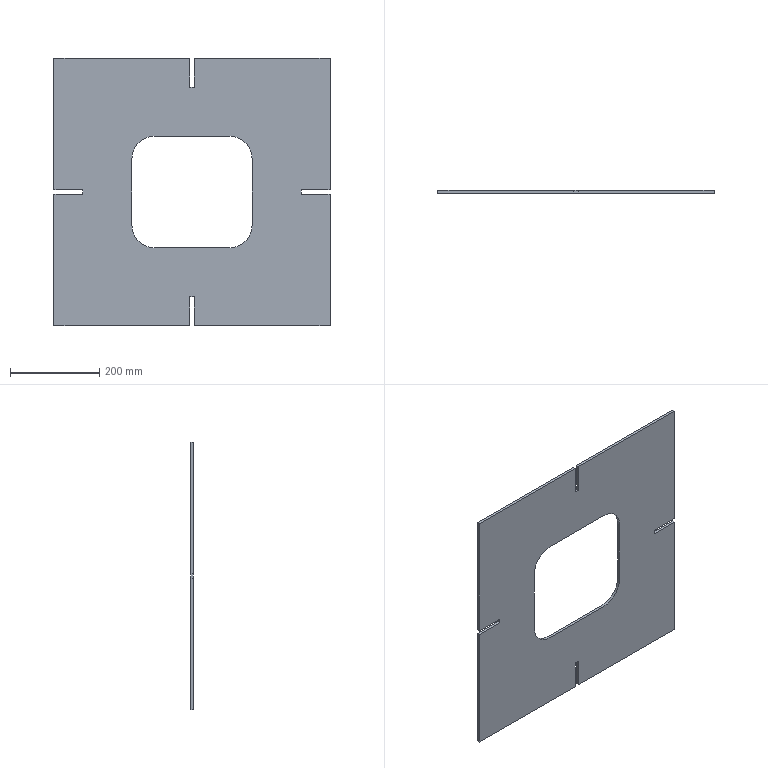Part | SolidWorks | features FlatPattern 1, SMBaseFlange 1, SheetMetal 1 | 1 solid | 30 faces | box 620 x 6 x 600 mm | volume 1824276 mm3 | plane 26 | cylinder 4 | commonest cylinder face diameters 100 x4
STEP:
#1=CARTESIAN_POINT('',(310.,0.,300.));
#2=VERTEX_POINT('',#1);
#3=CARTESIAN_POINT('',(310.,0.,5.));
#4=VERTEX_POINT('',#3);
#5=CARTESIAN_POINT('',(310.,0.,5.));
#6=DIRECTION('',(0.,0.,-1.));
#7=VECTOR('',#6,1000.);
#8=LINE('',#5,#7);
#9=EDGE_CURVE('',#2,#4,#8,.T.);
#10=ORIENTED_EDGE('',*,*,#9,.F.);
#11=CARTESIAN_POINT('',(310.,-6.,300.));
#12=VERTEX_POINT('',#11);
#13=CARTESIAN_POINT('',(310.,-6.,300.));
#14=DIRECTION('',(0.,1.,0.));
#15=VECTOR('',#14,1000.);
#16=LINE('',#13,#15);
#17=EDGE_CURVE('',#12,#2,#16,.T.);
#18=ORIENTED_EDGE('',*,*,#17,.F.);
#19=CARTESIAN_POINT('',(310.,-6.,5.));
#20=VERTEX_POINT('',#19);
#21=CARTESIAN_POINT('',(310.,-6.,5.));
#22=DIRECTION('',(0.,0.,-1.));
#23=VECTOR('',#22,1000.);
#24=LINE('',#21,#23);
#25=EDGE_CURVE('',#12,#20,#24,.T.);
#26=ORIENTED_EDGE('',*,*,#25,.T.);
#27=CARTESIAN_POINT('',(310.,-6.,5.));
#28=DIRECTION('',(0.,1.,0.));
#29=VECTOR('',#28,1000.);
#30=LINE('',#27,#29);
#31=EDGE_CURVE('',#20,#4,#30,.T.);
#32=ORIENTED_EDGE('',*,*,#31,.T.);
#33=EDGE_LOOP('',(#10,#18,#26,#32));
#34=FACE_OUTER_BOUND('',#33,.T.);
#35=CARTESIAN_POINT('',(310.,-6.,5.));
#36=DIRECTION('',(1.,0.,0.));
#37=DIRECTION('',(0.,0.,-1.));
#38=AXIS2_PLACEMENT_3D('',#35,#36,#37);
#39=PLANE('',#38);
#40=ADVANCED_FACE('',(#34),#39,.T.);
#41=CARTESIAN_POINT('',(5.,0.,300.));
#42=VERTEX_POINT('',#41);
#43=CARTESIAN_POINT('',(5.,0.,300.));
#44=DIRECTION('',(1.,0.,0.));
#45=VECTOR('',#44,1000.);
#46=LINE('',#43,#45);
#47=EDGE_CURVE('',#42,#2,#46,.T.);
#48=ORIENTED_EDGE('',*,*,#47,.F.);
#49=CARTESIAN_POINT('',(5.,-6.,300.));
#50=VERTEX_POINT('',#49);
#51=CARTESIAN_POINT('',(5.,-6.,300.));
#52=DIRECTION('',(0.,1.,0.));
#53=VECTOR('',#52,1000.);
#54=LINE('',#51,#53);
#55=EDGE_CURVE('',#50,#42,#54,.T.);
#56=ORIENTED_EDGE('',*,*,#55,.F.);
#57=CARTESIAN_POINT('',(5.,-6.,300.));
#58=DIRECTION('',(1.,0.,0.));
#59=VECTOR('',#58,1000.);
#60=LINE('',#57,#59);
#61=EDGE_CURVE('',#50,#12,#60,.T.);
#62=ORIENTED_EDGE('',*,*,#61,.T.);
#63=ORIENTED_EDGE('',*,*,#17,.T.);
#64=EDGE_LOOP('',(#48,#56,#62,#63));
#65=FACE_OUTER_BOUND('',#64,.T.);
#66=CARTESIAN_POINT('',(5.,-6.,300.));
#67=DIRECTION('',(0.,0.,1.));
#68=DIRECTION('',(1.,0.,0.));
#69=AXIS2_PLACEMENT_3D('',#66,#67,#68);
#70=PLANE('',#69);
#71=ADVANCED_FACE('',(#65),#70,.T.);
#72=CARTESIAN_POINT('',(5.,0.,235.));
#73=VERTEX_POINT('',#72);
#74=CARTESIAN_POINT('',(5.,0.,300.));
#75=DIRECTION('',(0.,0.,1.));
#76=VECTOR('',#75,1000.);
#77=LINE('',#74,#76);
#78=EDGE_CURVE('',#73,#42,#77,.T.);
#79=ORIENTED_EDGE('',*,*,#78,.F.);
#80=CARTESIAN_POINT('',(5.,-6.,235.));
#81=VERTEX_POINT('',#80);
#82=CARTESIAN_POINT('',(5.,-6.,235.));
#83=DIRECTION('',(0.,1.,0.));
#84=VECTOR('',#83,1000.);
#85=LINE('',#82,#84);
#86=EDGE_CURVE('',#81,#73,#85,.T.);
#87=ORIENTED_EDGE('',*,*,#86,.F.);
#88=CARTESIAN_POINT('',(5.,-6.,300.));
#89=DIRECTION('',(0.,0.,1.));
#90=VECTOR('',#89,1000.);
#91=LINE('',#88,#90);
#92=EDGE_CURVE('',#81,#50,#91,.T.);
#93=ORIENTED_EDGE('',*,*,#92,.T.);
#94=ORIENTED_EDGE('',*,*,#55,.T.);
#95=EDGE_LOOP('',(#79,#87,#93,#94));
#96=FACE_OUTER_BOUND('',#95,.T.);
#97=CARTESIAN_POINT('',(5.,-6.,300.));
#98=DIRECTION('',(-1.,0.,0.));
#99=DIRECTION('',(0.,0.,1.));
#100=AXIS2_PLACEMENT_3D('',#97,#98,#99);
#101=PLANE('',#100);
#102=ADVANCED_FACE('',(#96),#101,.T.);
#103=CARTESIAN_POINT('',(-5.,0.,235.));
#104=VERTEX_POINT('',#103);
#105=CARTESIAN_POINT('',(5.,0.,235.));
#106=DIRECTION('',(1.,0.,0.));
#107=VECTOR('',#106,1000.);
#108=LINE('',#105,#107);
#109=EDGE_CURVE('',#104,#73,#108,.T.);
#110=ORIENTED_EDGE('',*,*,#109,.F.);
#111=CARTESIAN_POINT('',(-5.,-6.,235.));
#112=VERTEX_POINT('',#111);
#113=CARTESIAN_POINT('',(-5.,-6.,235.));
#114=DIRECTION('',(0.,1.,0.));
#115=VECTOR('',#114,1000.);
#116=LINE('',#113,#115);
#117=EDGE_CURVE('',#112,#104,#116,.T.);
#118=ORIENTED_EDGE('',*,*,#117,.F.);
#119=CARTESIAN_POINT('',(5.,-6.,235.));
#120=DIRECTION('',(1.,0.,0.));
#121=VECTOR('',#120,1000.);
#122=LINE('',#119,#121);
#123=EDGE_CURVE('',#112,#81,#122,.T.);
#124=ORIENTED_EDGE('',*,*,#123,.T.);
#125=ORIENTED_EDGE('',*,*,#86,.T.);
#126=EDGE_LOOP('',(#110,#118,#124,#125));
#127=FACE_OUTER_BOUND('',#126,.T.);
#128=CARTESIAN_POINT('',(5.,-6.,235.));
#129=DIRECTION('',(0.,0.,1.));
#130=DIRECTION('',(1.,0.,0.));
#131=AXIS2_PLACEMENT_3D('',#128,#129,#130);
#132=PLANE('',#131);
#133=ADVANCED_FACE('',(#127),#132,.T.);
#134=CARTESIAN_POINT('',(-5.,0.,300.));
#135=VERTEX_POINT('',#134);
#136=CARTESIAN_POINT('',(-5.,0.,235.));
#137=DIRECTION('',(0.,0.,-1.));
#138=VECTOR('',#137,1000.);
#139=LINE('',#136,#138);
#140=EDGE_CURVE('',#135,#104,#139,.T.);
#141=ORIENTED_EDGE('',*,*,#140,.F.);
#142=CARTESIAN_POINT('',(-5.,-6.,300.));
#143=VERTEX_POINT('',#142);
#144=CARTESIAN_POINT('',(-5.,-6.,300.));
#145=DIRECTION('',(0.,1.,0.));
#146=VECTOR('',#145,1000.);
#147=LINE('',#144,#146);
#148=EDGE_CURVE('',#143,#135,#147,.T.);
#149=ORIENTED_EDGE('',*,*,#148,.F.);
#150=CARTESIAN_POINT('',(-5.,-6.,235.));
#151=DIRECTION('',(0.,0.,-1.));
#152=VECTOR('',#151,1000.);
#153=LINE('',#150,#152);
#154=EDGE_CURVE('',#143,#112,#153,.T.);
#155=ORIENTED_EDGE('',*,*,#154,.T.);
#156=ORIENTED_EDGE('',*,*,#117,.T.);
#157=EDGE_LOOP('',(#141,#149,#155,#156));
#158=FACE_OUTER_BOUND('',#157,.T.);
#159=CARTESIAN_POINT('',(-5.,-6.,235.));
#160=DIRECTION('',(1.,0.,0.));
#161=DIRECTION('',(0.,0.,-1.));
#162=AXIS2_PLACEMENT_3D('',#159,#160,#161);
#163=PLANE('',#162);
#164=ADVANCED_FACE('',(#158),#163,.T.);
#165=CARTESIAN_POINT('',(-310.,0.,300.));
#166=VERTEX_POINT('',#165);
#167=CARTESIAN_POINT('',(-310.,0.,300.));
#168=DIRECTION('',(1.,0.,0.));
#169=VECTOR('',#168,1000.);
#170=LINE('',#167,#169);
#171=EDGE_CURVE('',#166,#135,#170,.T.);
#172=ORIENTED_EDGE('',*,*,#171,.F.);
#173=CARTESIAN_POINT('',(-310.,-6.,300.));
#174=VERTEX_POINT('',#173);
#175=CARTESIAN_POINT('',(-310.,-6.,300.));
#176=DIRECTION('',(0.,1.,0.));
#177=VECTOR('',#176,1000.);
#178=LINE('',#175,#177);
#179=EDGE_CURVE('',#174,#166,#178,.T.);
#180=ORIENTED_EDGE('',*,*,#179,.F.);
#181=CARTESIAN_POINT('',(-310.,-6.,300.));
#182=DIRECTION('',(1.,0.,0.));
#183=VECTOR('',#182,1000.);
#184=LINE('',#181,#183);
#185=EDGE_CURVE('',#174,#143,#184,.T.);
#186=ORIENTED_EDGE('',*,*,#185,.T.);
#187=ORIENTED_EDGE('',*,*,#148,.T.);
#188=EDGE_LOOP('',(#172,#180,#186,#187));
#189=FACE_OUTER_BOUND('',#188,.T.);
#190=CARTESIAN_POINT('',(-310.,-6.,300.));
#191=DIRECTION('',(0.,0.,1.));
#192=DIRECTION('',(1.,0.,0.));
#193=AXIS2_PLACEMENT_3D('',#190,#191,#192);
#194=PLANE('',#193);
#195=ADVANCED_FACE('',(#189),#194,.T.);
#196=CARTESIAN_POINT('',(-310.,0.,5.));
#197=VERTEX_POINT('',#196);
#198=CARTESIAN_POINT('',(-310.,0.,5.));
#199=DIRECTION('',(0.,0.,1.));
#200=VECTOR('',#199,1000.);
#201=LINE('',#198,#200);
#202=EDGE_CURVE('',#197,#166,#201,.T.);
#203=ORIENTED_EDGE('',*,*,#202,.F.);
#204=CARTESIAN_POINT('',(-310.,-6.,5.));
#205=VERTEX_POINT('',#204);
#206=CARTESIAN_POINT('',(-310.,-6.,5.));
#207=DIRECTION('',(0.,1.,0.));
#208=VECTOR('',#207,1000.);
#209=LINE('',#206,#208);
#210=EDGE_CURVE('',#205,#197,#209,.T.);
#211=ORIENTED_EDGE('',*,*,#210,.F.);
#212=CARTESIAN_POINT('',(-310.,-6.,5.));
#213=DIRECTION('',(0.,0.,1.));
#214=VECTOR('',#213,1000.);
#215=LINE('',#212,#214);
#216=EDGE_CURVE('',#205,#174,#215,.T.);
#217=ORIENTED_EDGE('',*,*,#216,.T.);
#218=ORIENTED_EDGE('',*,*,#179,.T.);
#219=EDGE_LOOP('',(#203,#211,#217,#218));
#220=FACE_OUTER_BOUND('',#219,.T.);
#221=CARTESIAN_POINT('',(-310.,-6.,5.));
#222=DIRECTION('',(-1.,0.,0.));
#223=DIRECTION('',(0.,0.,1.));
#224=AXIS2_PLACEMENT_3D('',#221,#222,#223);
#225=PLANE('',#224);
#226=ADVANCED_FACE('',(#220),#225,.T.);
#227=CARTESIAN_POINT('',(-245.,0.,5.));
#228=VERTEX_POINT('',#227);
#229=CARTESIAN_POINT('',(-245.,0.,5.));
#230=DIRECTION('',(-1.,0.,0.));
#231=VECTOR('',#230,1000.);
#232=LINE('',#229,#231);
#233=EDGE_CURVE('',#228,#197,#232,.T.);
#234=ORIENTED_EDGE('',*,*,#233,.F.);
#235=CARTESIAN_POINT('',(-245.,-6.,5.));
#236=VERTEX_POINT('',#235);
#237=CARTESIAN_POINT('',(-245.,-6.,5.));
#238=DIRECTION('',(0.,1.,0.));
#239=VECTOR('',#238,1000.);
#240=LINE('',#237,#239);
#241=EDGE_CURVE('',#236,#228,#240,.T.);
#242=ORIENTED_EDGE('',*,*,#241,.F.);
#243=CARTESIAN_POINT('',(-245.,-6.,5.));
#244=DIRECTION('',(-1.,0.,0.));
#245=VECTOR('',#244,1000.);
#246=LINE('',#243,#245);
#247=EDGE_CURVE('',#236,#205,#246,.T.);
#248=ORIENTED_EDGE('',*,*,#247,.T.);
#249=ORIENTED_EDGE('',*,*,#210,.T.);
#250=EDGE_LOOP('',(#234,#242,#248,#249));
#251=FACE_OUTER_BOUND('',#250,.T.);
#252=CARTESIAN_POINT('',(-245.,-6.,5.));
#253=DIRECTION('',(0.,0.,-1.));
#254=DIRECTION('',(-1.,0.,0.));
#255=AXIS2_PLACEMENT_3D('',#252,#253,#254);
#256=PLANE('',#255);
#257=ADVANCED_FACE('',(#251),#256,.T.);
#258=CARTESIAN_POINT('',(-245.,0.,-5.));
#259=VERTEX_POINT('',#258);
#260=CARTESIAN_POINT('',(-245.,0.,-5.));
#261=DIRECTION('',(0.,0.,1.));
#262=VECTOR('',#261,1000.);
#263=LINE('',#260,#262);
#264=EDGE_CURVE('',#259,#228,#263,.T.);
#265=ORIENTED_EDGE('',*,*,#264,.F.);
#266=CARTESIAN_POINT('',(-245.,-6.,-5.));
#267=VERTEX_POINT('',#266);
#268=CARTESIAN_POINT('',(-245.,-6.,-5.));
#269=DIRECTION('',(0.,1.,0.));
#270=VECTOR('',#269,1000.);
#271=LINE('',#268,#270);
#272=EDGE_CURVE('',#267,#259,#271,.T.);
#273=ORIENTED_EDGE('',*,*,#272,.F.);
#274=CARTESIAN_POINT('',(-245.,-6.,-5.));
#275=DIRECTION('',(0.,0.,1.));
#276=VECTOR('',#275,1000.);
#277=LINE('',#274,#276);
#278=EDGE_CURVE('',#267,#236,#277,.T.);
#279=ORIENTED_EDGE('',*,*,#278,.T.);
#280=ORIENTED_EDGE('',*,*,#241,.T.);
#281=EDGE_LOOP('',(#265,#273,#279,#280));
#282=FACE_OUTER_BOUND('',#281,.T.);
#283=CARTESIAN_POINT('',(-245.,-6.,-5.));
#284=DIRECTION('',(-1.,0.,0.));
#285=DIRECTION('',(0.,0.,1.));
#286=AXIS2_PLACEMENT_3D('',#283,#284,#285);
#287=PLANE('',#286);
#288=ADVANCED_FACE('',(#282),#287,.T.);
#289=CARTESIAN_POINT('',(-310.,0.,-5.));
#290=VERTEX_POINT('',#289);
#291=CARTESIAN_POINT('',(-310.,0.,-5.));
#292=DIRECTION('',(1.,0.,0.));
#293=VECTOR('',#292,1000.);
#294=LINE('',#291,#293);
#295=EDGE_CURVE('',#290,#259,#294,.T.);
#296=ORIENTED_EDGE('',*,*,#295,.F.);
#297=CARTESIAN_POINT('',(-310.,-6.,-5.));
#298=VERTEX_POINT('',#297);
#299=CARTESIAN_POINT('',(-310.,-6.,-5.));
#300=DIRECTION('',(0.,1.,0.));
#301=VECTOR('',#300,1000.);
#302=LINE('',#299,#301);
#303=EDGE_CURVE('',#298,#290,#302,.T.);
#304=ORIENTED_EDGE('',*,*,#303,.F.);
#305=CARTESIAN_POINT('',(-310.,-6.,-5.));
#306=DIRECTION('',(1.,0.,0.));
#307=VECTOR('',#306,1000.);
#308=LINE('',#305,#307);
#309=EDGE_CURVE('',#298,#267,#308,.T.);
#310=ORIENTED_EDGE('',*,*,#309,.T.);
#311=ORIENTED_EDGE('',*,*,#272,.T.);
#312=EDGE_LOOP('',(#296,#304,#310,#311));
#313=FACE_OUTER_BOUND('',#312,.T.);
#314=CARTESIAN_POINT('',(-310.,-6.,-5.));
#315=DIRECTION('',(0.,0.,1.));
#316=DIRECTION('',(1.,0.,0.));
#317=AXIS2_PLACEMENT_3D('',#314,#315,#316);
#318=PLANE('',#317);
#319=ADVANCED_FACE('',(#313),#318,.T.);
#320=CARTESIAN_POINT('',(-310.,0.,-300.));
#321=VERTEX_POINT('',#320);
#322=CARTESIAN_POINT('',(-310.,0.,-300.));
#323=DIRECTION('',(0.,0.,1.));
#324=VECTOR('',#323,1000.);
#325=LINE('',#322,#324);
#326=EDGE_CURVE('',#321,#290,#325,.T.);
#327=ORIENTED_EDGE('',*,*,#326,.F.);
#328=CARTESIAN_POINT('',(-310.,-6.,-300.));
#329=VERTEX_POINT('',#328);
#330=CARTESIAN_POINT('',(-310.,-6.,-300.));
#331=DIRECTION('',(0.,1.,0.));
#332=VECTOR('',#331,1000.);
#333=LINE('',#330,#332);
#334=EDGE_CURVE('',#329,#321,#333,.T.);
#335=ORIENTED_EDGE('',*,*,#334,.F.);
#336=CARTESIAN_POINT('',(-310.,-6.,-300.));
#337=DIRECTION('',(0.,0.,1.));
#338=VECTOR('',#337,1000.);
#339=LINE('',#336,#338);
#340=EDGE_CURVE('',#329,#298,#339,.T.);
#341=ORIENTED_EDGE('',*,*,#340,.T.);
#342=ORIENTED_EDGE('',*,*,#303,.T.);
#343=EDGE_LOOP('',(#327,#335,#341,#342));
#344=FACE_OUTER_BOUND('',#343,.T.);
#345=CARTESIAN_POINT('',(-310.,-6.,-300.));
#346=DIRECTION('',(-1.,0.,0.));
#347=DIRECTION('',(0.,0.,1.));
#348=AXIS2_PLACEMENT_3D('',#345,#346,#347);
#349=PLANE('',#348);
#350=ADVANCED_FACE('',(#344),#349,.T.);
#351=CARTESIAN_POINT('',(-5.,0.,-300.));
#352=VERTEX_POINT('',#351);
#353=CARTESIAN_POINT('',(-310.,0.,-300.));
#354=DIRECTION('',(-1.,0.,0.));
#355=VECTOR('',#354,1000.);
#356=LINE('',#353,#355);
#357=EDGE_CURVE('',#352,#321,#356,.T.);
#358=ORIENTED_EDGE('',*,*,#357,.F.);
#359=CARTESIAN_POINT('',(-5.,-6.,-300.));
#360=VERTEX_POINT('',#359);
#361=CARTESIAN_POINT('',(-5.,-6.,-300.));
#362=DIRECTION('',(0.,1.,0.));
#363=VECTOR('',#362,1000.);
#364=LINE('',#361,#363);
#365=EDGE_CURVE('',#360,#352,#364,.T.);
#366=ORIENTED_EDGE('',*,*,#365,.F.);
#367=CARTESIAN_POINT('',(-310.,-6.,-300.));
#368=DIRECTION('',(-1.,0.,0.));
#369=VECTOR('',#368,1000.);
#370=LINE('',#367,#369);
#371=EDGE_CURVE('',#360,#329,#370,.T.);
#372=ORIENTED_EDGE('',*,*,#371,.T.);
#373=ORIENTED_EDGE('',*,*,#334,.T.);
#374=EDGE_LOOP('',(#358,#366,#372,#373));
#375=FACE_OUTER_BOUND('',#374,.T.);
#376=CARTESIAN_POINT('',(-310.,-6.,-300.));
#377=DIRECTION('',(0.,0.,-1.));
#378=DIRECTION('',(-1.,0.,0.));
#379=AXIS2_PLACEMENT_3D('',#376,#377,#378);
#380=PLANE('',#379);
#381=ADVANCED_FACE('',(#375),#380,.T.);
#382=CARTESIAN_POINT('',(-5.,0.,-235.));
#383=VERTEX_POINT('',#382);
#384=CARTESIAN_POINT('',(-5.,0.,-235.));
#385=DIRECTION('',(0.,0.,-1.));
#386=VECTOR('',#385,1000.);
#387=LINE('',#384,#386);
#388=EDGE_CURVE('',#383,#352,#387,.T.);
#389=ORIENTED_EDGE('',*,*,#388,.F.);
#390=CARTESIAN_POINT('',(-5.,-6.,-235.));
#391=VERTEX_POINT('',#390);
#392=CARTESIAN_POINT('',(-5.,-6.,-235.));
#393=DIRECTION('',(0.,1.,0.));
#394=VECTOR('',#393,1000.);
#395=LINE('',#392,#394);
#396=EDGE_CURVE('',#391,#383,#395,.T.);
#397=ORIENTED_EDGE('',*,*,#396,.F.);
#398=CARTESIAN_POINT('',(-5.,-6.,-235.));
#399=DIRECTION('',(0.,0.,-1.));
#400=VECTOR('',#399,1000.);
#401=LINE('',#398,#400);
#402=EDGE_CURVE('',#391,#360,#401,.T.);
#403=ORIENTED_EDGE('',*,*,#402,.T.);
#404=ORIENTED_EDGE('',*,*,#365,.T.);
#405=EDGE_LOOP('',(#389,#397,#403,#404));
#406=FACE_OUTER_BOUND('',#405,.T.);
#407=CARTESIAN_POINT('',(-5.,-6.,-235.));
#408=DIRECTION('',(1.,0.,0.));
#409=DIRECTION('',(0.,0.,-1.));
#410=AXIS2_PLACEMENT_3D('',#407,#408,#409);
#411=PLANE('',#410);
#412=ADVANCED_FACE('',(#406),#411,.T.);
#413=CARTESIAN_POINT('',(5.,0.,-235.));
#414=VERTEX_POINT('',#413);
#415=CARTESIAN_POINT('',(5.,0.,-235.));
#416=DIRECTION('',(-1.,0.,0.));
#417=VECTOR('',#416,1000.);
#418=LINE('',#415,#417);
#419=EDGE_CURVE('',#414,#383,#418,.T.);
#420=ORIENTED_EDGE('',*,*,#419,.F.);
#421=CARTESIAN_POINT('',(5.,-6.,-235.));
#422=VERTEX_POINT('',#421);
#423=CARTESIAN_POINT('',(5.,-6.,-235.));
#424=DIRECTION('',(0.,1.,0.));
#425=VECTOR('',#424,1000.);
#426=LINE('',#423,#425);
#427=EDGE_CURVE('',#422,#414,#426,.T.);
#428=ORIENTED_EDGE('',*,*,#427,.F.);
#429=CARTESIAN_POINT('',(5.,-6.,-235.));
#430=DIRECTION('',(-1.,0.,0.));
#431=VECTOR('',#430,1000.);
#432=LINE('',#429,#431);
#433=EDGE_CURVE('',#422,#391,#432,.T.);
#434=ORIENTED_EDGE('',*,*,#433,.T.);
#435=ORIENTED_EDGE('',*,*,#396,.T.);
#436=EDGE_LOOP('',(#420,#428,#434,#435));
#437=FACE_OUTER_BOUND('',#436,.T.);
#438=CARTESIAN_POINT('',(5.,-6.,-235.));
#439=DIRECTION('',(0.,0.,-1.));
#440=DIRECTION('',(-1.,0.,0.));
#441=AXIS2_PLACEMENT_3D('',#438,#439,#440);
#442=PLANE('',#441);
#443=ADVANCED_FACE('',(#437),#442,.T.);
#444=CARTESIAN_POINT('',(5.,0.,-300.));
#445=VERTEX_POINT('',#444);
#446=CARTESIAN_POINT('',(5.,0.,-300.));
#447=DIRECTION('',(0.,0.,1.));
#448=VECTOR('',#447,1000.);
#449=LINE('',#446,#448);
#450=EDGE_CURVE('',#445,#414,#449,.T.);
#451=ORIENTED_EDGE('',*,*,#450,.F.);
#452=CARTESIAN_POINT('',(5.,-6.,-300.));
#453=VERTEX_POINT('',#452);
#454=CARTESIAN_POINT('',(5.,-6.,-300.));
#455=DIRECTION('',(0.,1.,0.));
#456=VECTOR('',#455,1000.);
#457=LINE('',#454,#456);
#458=EDGE_CURVE('',#453,#445,#457,.T.);
#459=ORIENTED_EDGE('',*,*,#458,.F.);
#460=CARTESIAN_POINT('',(5.,-6.,-300.));
#461=DIRECTION('',(0.,0.,1.));
#462=VECTOR('',#461,1000.);
#463=LINE('',#460,#462);
#464=EDGE_CURVE('',#453,#422,#463,.T.);
#465=ORIENTED_EDGE('',*,*,#464,.T.);
#466=ORIENTED_EDGE('',*,*,#427,.T.);
#467=EDGE_LOOP('',(#451,#459,#465,#466));
#468=FACE_OUTER_BOUND('',#467,.T.);
#469=CARTESIAN_POINT('',(5.,-6.,-300.));
#470=DIRECTION('',(-1.,0.,0.));
#471=DIRECTION('',(0.,0.,1.));
#472=AXIS2_PLACEMENT_3D('',#469,#470,#471);
#473=PLANE('',#472);
#474=ADVANCED_FACE('',(#468),#473,.T.);
#475=CARTESIAN_POINT('',(310.,0.,-300.));
#476=VERTEX_POINT('',#475);
#477=CARTESIAN_POINT('',(5.,0.,-300.));
#478=DIRECTION('',(-1.,0.,0.));
#479=VECTOR('',#478,1000.);
#480=LINE('',#477,#479);
#481=EDGE_CURVE('',#476,#445,#480,.T.);
#482=ORIENTED_EDGE('',*,*,#481,.F.);
#483=CARTESIAN_POINT('',(310.,-6.,-300.));
#484=VERTEX_POINT('',#483);
#485=CARTESIAN_POINT('',(310.,-6.,-300.));
#486=DIRECTION('',(0.,1.,0.));
#487=VECTOR('',#486,1000.);
#488=LINE('',#485,#487);
#489=EDGE_CURVE('',#484,#476,#488,.T.);
#490=ORIENTED_EDGE('',*,*,#489,.F.);
#491=CARTESIAN_POINT('',(5.,-6.,-300.));
#492=DIRECTION('',(-1.,0.,0.));
#493=VECTOR('',#492,1000.);
#494=LINE('',#491,#493);
#495=EDGE_CURVE('',#484,#453,#494,.T.);
#496=ORIENTED_EDGE('',*,*,#495,.T.);
#497=ORIENTED_EDGE('',*,*,#458,.T.);
#498=EDGE_LOOP('',(#482,#490,#496,#497));
#499=FACE_OUTER_BOUND('',#498,.T.);
#500=CARTESIAN_POINT('',(5.,-6.,-300.));
#501=DIRECTION('',(0.,0.,-1.));
#502=DIRECTION('',(-1.,0.,0.));
#503=AXIS2_PLACEMENT_3D('',#500,#501,#502);
#504=PLANE('',#503);
#505=ADVANCED_FACE('',(#499),#504,.T.);
#506=CARTESIAN_POINT('',(310.,0.,-5.));
#507=VERTEX_POINT('',#506);
#508=CARTESIAN_POINT('',(310.,0.,-300.));
#509=DIRECTION('',(0.,0.,-1.));
#510=VECTOR('',#509,1000.);
#511=LINE('',#508,#510);
#512=EDGE_CURVE('',#507,#476,#511,.T.);
#513=ORIENTED_EDGE('',*,*,#512,.F.);
#514=CARTESIAN_POINT('',(310.,-6.,-5.));
#515=VERTEX_POINT('',#514);
#516=CARTESIAN_POINT('',(310.,-6.,-5.));
#517=DIRECTION('',(0.,1.,0.));
#518=VECTOR('',#517,1000.);
#519=LINE('',#516,#518);
#520=EDGE_CURVE('',#515,#507,#519,.T.);
#521=ORIENTED_EDGE('',*,*,#520,.F.);
#522=CARTESIAN_POINT('',(310.,-6.,-300.));
#523=DIRECTION('',(0.,0.,-1.));
#524=VECTOR('',#523,1000.);
#525=LINE('',#522,#524);
#526=EDGE_CURVE('',#515,#484,#525,.T.);
#527=ORIENTED_EDGE('',*,*,#526,.T.);
#528=ORIENTED_EDGE('',*,*,#489,.T.);
#529=EDGE_LOOP('',(#513,#521,#527,#528));
#530=FACE_OUTER_BOUND('',#529,.T.);
#531=CARTESIAN_POINT('',(310.,-6.,-300.));
#532=DIRECTION('',(1.,0.,0.));
#533=DIRECTION('',(0.,0.,-1.));
#534=AXIS2_PLACEMENT_3D('',#531,#532,#533);
#535=PLANE('',#534);
#536=ADVANCED_FACE('',(#530),#535,.T.);
#537=CARTESIAN_POINT('',(245.,0.,-5.));
#538=VERTEX_POINT('',#537);
#539=CARTESIAN_POINT('',(310.,0.,-5.));
#540=DIRECTION('',(1.,0.,0.));
#541=VECTOR('',#540,1000.);
#542=LINE('',#539,#541);
#543=EDGE_CURVE('',#538,#507,#542,.T.);
#544=ORIENTED_EDGE('',*,*,#543,.F.);
#545=CARTESIAN_POINT('',(245.,-6.,-5.));
#546=VERTEX_POINT('',#545);
#547=CARTESIAN_POINT('',(245.,-6.,-5.));
#548=DIRECTION('',(0.,1.,0.));
#549=VECTOR('',#548,1000.);
#550=LINE('',#547,#549);
#551=EDGE_CURVE('',#546,#538,#550,.T.);
#552=ORIENTED_EDGE('',*,*,#551,.F.);
#553=CARTESIAN_POINT('',(310.,-6.,-5.));
#554=DIRECTION('',(1.,0.,0.));
#555=VECTOR('',#554,1000.);
#556=LINE('',#553,#555);
#557=EDGE_CURVE('',#546,#515,#556,.T.);
#558=ORIENTED_EDGE('',*,*,#557,.T.);
#559=ORIENTED_EDGE('',*,*,#520,.T.);
#560=EDGE_LOOP('',(#544,#552,#558,#559));
#561=FACE_OUTER_BOUND('',#560,.T.);
#562=CARTESIAN_POINT('',(310.,-6.,-5.));
#563=DIRECTION('',(0.,0.,1.));
#564=DIRECTION('',(1.,0.,0.));
#565=AXIS2_PLACEMENT_3D('',#562,#563,#564);
#566=PLANE('',#565);
#567=ADVANCED_FACE('',(#561),#566,.T.);
#568=CARTESIAN_POINT('',(245.,0.,5.));
#569=VERTEX_POINT('',#568);
#570=CARTESIAN_POINT('',(245.,0.,-5.));
#571=DIRECTION('',(0.,0.,-1.));
#572=VECTOR('',#571,1000.);
#573=LINE('',#570,#572);
#574=EDGE_CURVE('',#569,#538,#573,.T.);
#575=ORIENTED_EDGE('',*,*,#574,.F.);
#576=CARTESIAN_POINT('',(245.,-6.,5.));
#577=VERTEX_POINT('',#576);
#578=CARTESIAN_POINT('',(245.,-6.,5.));
#579=DIRECTION('',(0.,1.,0.));
#580=VECTOR('',#579,1000.);
#581=LINE('',#578,#580);
#582=EDGE_CURVE('',#577,#569,#581,.T.);
#583=ORIENTED_EDGE('',*,*,#582,.F.);
#584=CARTESIAN_POINT('',(245.,-6.,-5.));
#585=DIRECTION('',(0.,0.,-1.));
#586=VECTOR('',#585,1000.);
#587=LINE('',#584,#586);
#588=EDGE_CURVE('',#577,#546,#587,.T.);
#589=ORIENTED_EDGE('',*,*,#588,.T.);
#590=ORIENTED_EDGE('',*,*,#551,.T.);
#591=EDGE_LOOP('',(#575,#583,#589,#590));
#592=FACE_OUTER_BOUND('',#591,.T.);
#593=CARTESIAN_POINT('',(245.,-6.,-5.));
#594=DIRECTION('',(1.,0.,0.));
#595=DIRECTION('',(0.,0.,-1.));
#596=AXIS2_PLACEMENT_3D('',#593,#594,#595);
#597=PLANE('',#596);
#598=ADVANCED_FACE('',(#592),#597,.T.);
#599=CARTESIAN_POINT('',(245.,0.,5.));
#600=DIRECTION('',(-1.,0.,0.));
#601=VECTOR('',#600,1000.);
#602=LINE('',#599,#601);
#603=EDGE_CURVE('',#4,#569,#602,.T.);
#604=ORIENTED_EDGE('',*,*,#603,.F.);
#605=ORIENTED_EDGE('',*,*,#31,.F.);
#606=CARTESIAN_POINT('',(245.,-6.,5.));
#607=DIRECTION('',(-1.,0.,0.));
#608=VECTOR('',#607,1000.);
#609=LINE('',#606,#608);
#610=EDGE_CURVE('',#20,#577,#609,.T.);
#611=ORIENTED_EDGE('',*,*,#610,.T.);
#612=ORIENTED_EDGE('',*,*,#582,.T.);
#613=EDGE_LOOP('',(#604,#605,#611,#612));
#614=FACE_OUTER_BOUND('',#613,.T.);
#615=CARTESIAN_POINT('',(245.,-6.,5.));
#616=DIRECTION('',(0.,0.,-1.));
#617=DIRECTION('',(-1.,0.,0.));
#618=AXIS2_PLACEMENT_3D('',#615,#616,#617);
#619=PLANE('',#618);
#620=ADVANCED_FACE('',(#614),#619,.T.);
#621=CARTESIAN_POINT('',(-135.,-6.,-75.));
#622=VERTEX_POINT('',#621);
#623=CARTESIAN_POINT('',(-135.,-6.,75.));
#624=VERTEX_POINT('',#623);
#625=CARTESIAN_POINT('',(-135.,-6.,-75.));
#626=DIRECTION('',(0.,0.,1.));
#627=VECTOR('',#626,1000.);
#628=LINE('',#625,#627);
#629=EDGE_CURVE('',#622,#624,#628,.T.);
#630=ORIENTED_EDGE('',*,*,#629,.T.);
#631=CARTESIAN_POINT('',(-85.,-6.,125.));
#632=VERTEX_POINT('',#631);
#633=CARTESIAN_POINT('',(-85.,-6.,75.));
#634=DIRECTION('',(0.,1.,0.));
#635=DIRECTION('',(0.,0.,1.));
#636=AXIS2_PLACEMENT_3D('',#633,#634,#635);
#637=CIRCLE('',#636,50.);
#638=EDGE_CURVE('',#624,#632,#637,.T.);
#639=ORIENTED_EDGE('',*,*,#638,.T.);
#640=CARTESIAN_POINT('',(85.,-6.,125.));
#641=VERTEX_POINT('',#640);
#642=CARTESIAN_POINT('',(-85.,-6.,125.));
#643=DIRECTION('',(1.,0.,0.));
#644=VECTOR('',#643,1000.);
#645=LINE('',#642,#644);
#646=EDGE_CURVE('',#632,#641,#645,.T.);
#647=ORIENTED_EDGE('',*,*,#646,.T.);
#648=CARTESIAN_POINT('',(135.,-6.,75.));
#649=VERTEX_POINT('',#648);
#650=CARTESIAN_POINT('',(85.,-6.,75.));
#651=DIRECTION('',(0.,1.,0.));
#652=DIRECTION('',(0.,0.,1.));
#653=AXIS2_PLACEMENT_3D('',#650,#651,#652);
#654=CIRCLE('',#653,50.);
#655=EDGE_CURVE('',#641,#649,#654,.T.);
#656=ORIENTED_EDGE('',*,*,#655,.T.);
#657=CARTESIAN_POINT('',(135.,-6.,-75.));
#658=VERTEX_POINT('',#657);
#659=CARTESIAN_POINT('',(135.,-6.,-75.));
#660=DIRECTION('',(0.,0.,-1.));
#661=VECTOR('',#660,1000.);
#662=LINE('',#659,#661);
#663=EDGE_CURVE('',#649,#658,#662,.T.);
#664=ORIENTED_EDGE('',*,*,#663,.T.);
#665=CARTESIAN_POINT('',(85.,-6.,-125.));
#666=VERTEX_POINT('',#665);
#667=CARTESIAN_POINT('',(85.,-6.,-75.));
#668=DIRECTION('',(0.,1.,0.));
#669=DIRECTION('',(0.,0.,-1.));
#670=AXIS2_PLACEMENT_3D('',#667,#668,#669);
#671=CIRCLE('',#670,50.);
#672=EDGE_CURVE('',#658,#666,#671,.T.);
#673=ORIENTED_EDGE('',*,*,#672,.T.);
#674=CARTESIAN_POINT('',(-85.,-6.,-125.));
#675=VERTEX_POINT('',#674);
#676=CARTESIAN_POINT('',(-85.,-6.,-125.));
#677=DIRECTION('',(-1.,0.,0.));
#678=VECTOR('',#677,1000.);
#679=LINE('',#676,#678);
#680=EDGE_CURVE('',#666,#675,#679,.T.);
#681=ORIENTED_EDGE('',*,*,#680,.T.);
#682=CARTESIAN_POINT('',(-85.,-6.,-75.));
#683=DIRECTION('',(0.,1.,0.));
#684=DIRECTION('',(0.,0.,1.));
#685=AXIS2_PLACEMENT_3D('',#682,#683,#684);
#686=CIRCLE('',#685,50.);
#687=EDGE_CURVE('',#675,#622,#686,.T.);
#688=ORIENTED_EDGE('',*,*,#687,.T.);
#689=EDGE_LOOP('',(#630,#639,#647,#656,#664,#673,#681,#688));
#690=FACE_BOUND('',#689,.T.);
#691=ORIENTED_EDGE('',*,*,#25,.F.);
#692=ORIENTED_EDGE('',*,*,#61,.F.);
#693=ORIENTED_EDGE('',*,*,#92,.F.);
#694=ORIENTED_EDGE('',*,*,#123,.F.);
#695=ORIENTED_EDGE('',*,*,#154,.F.);
#696=ORIENTED_EDGE('',*,*,#185,.F.);
#697=ORIENTED_EDGE('',*,*,#216,.F.);
#698=ORIENTED_EDGE('',*,*,#247,.F.);
#699=ORIENTED_EDGE('',*,*,#278,.F.);
#700=ORIENTED_EDGE('',*,*,#309,.F.);
#701=ORIENTED_EDGE('',*,*,#340,.F.);
#702=ORIENTED_EDGE('',*,*,#371,.F.);
#703=ORIENTED_EDGE('',*,*,#402,.F.);
#704=ORIENTED_EDGE('',*,*,#433,.F.);
#705=ORIENTED_EDGE('',*,*,#464,.F.);
#706=ORIENTED_EDGE('',*,*,#495,.F.);
#707=ORIENTED_EDGE('',*,*,#526,.F.);
#708=ORIENTED_EDGE('',*,*,#557,.F.);
#709=ORIENTED_EDGE('',*,*,#588,.F.);
#710=ORIENTED_EDGE('',*,*,#610,.F.);
#711=EDGE_LOOP('',(#691,#692,#693,#694,#695,#696,#697,#698,#699,#700,#701,#702,#703,#704,#705,#706,#707,#708,#709,#710));
#712=FACE_OUTER_BOUND('',#711,.T.);
#713=CARTESIAN_POINT('',(0.,-6.,0.));
#714=DIRECTION('',(0.,1.,0.));
#715=DIRECTION('',(0.,0.,1.));
#716=AXIS2_PLACEMENT_3D('',#713,#714,#715);
#717=PLANE('',#716);
#718=ADVANCED_FACE('',(#690,#712),#717,.F.);
#719=CARTESIAN_POINT('',(-135.,0.,75.));
#720=VERTEX_POINT('',#719);
#721=CARTESIAN_POINT('',(-85.,0.,125.));
#722=VERTEX_POINT('',#721);
#723=CARTESIAN_POINT('',(-85.,0.,75.));
#724=DIRECTION('',(0.,1.,0.));
#725=DIRECTION('',(0.,0.,1.));
#726=AXIS2_PLACEMENT_3D('',#723,#724,#725);
#727=CIRCLE('',#726,50.);
#728=EDGE_CURVE('',#720,#722,#727,.T.);
#729=ORIENTED_EDGE('',*,*,#728,.F.);
#730=CARTESIAN_POINT('',(-135.,0.,-75.));
#731=VERTEX_POINT('',#730);
#732=CARTESIAN_POINT('',(-135.,0.,-75.));
#733=DIRECTION('',(0.,0.,1.));
#734=VECTOR('',#733,1000.);
#735=LINE('',#732,#734);
#736=EDGE_CURVE('',#731,#720,#735,.T.);
#737=ORIENTED_EDGE('',*,*,#736,.F.);
#738=CARTESIAN_POINT('',(-85.,0.,-125.));
#739=VERTEX_POINT('',#738);
#740=CARTESIAN_POINT('',(-85.,0.,-75.));
#741=DIRECTION('',(0.,1.,0.));
#742=DIRECTION('',(0.,0.,1.));
#743=AXIS2_PLACEMENT_3D('',#740,#741,#742);
#744=CIRCLE('',#743,50.);
#745=EDGE_CURVE('',#739,#731,#744,.T.);
#746=ORIENTED_EDGE('',*,*,#745,.F.);
#747=CARTESIAN_POINT('',(85.,0.,-125.));
#748=VERTEX_POINT('',#747);
#749=CARTESIAN_POINT('',(-85.,0.,-125.));
#750=DIRECTION('',(-1.,0.,0.));
#751=VECTOR('',#750,1000.);
#752=LINE('',#749,#751);
#753=EDGE_CURVE('',#748,#739,#752,.T.);
#754=ORIENTED_EDGE('',*,*,#753,.F.);
#755=CARTESIAN_POINT('',(135.,0.,-75.));
#756=VERTEX_POINT('',#755);
#757=CARTESIAN_POINT('',(85.,0.,-75.));
#758=DIRECTION('',(0.,1.,0.));
#759=DIRECTION('',(0.,0.,-1.));
#760=AXIS2_PLACEMENT_3D('',#757,#758,#759);
#761=CIRCLE('',#760,50.);
#762=EDGE_CURVE('',#756,#748,#761,.T.);
#763=ORIENTED_EDGE('',*,*,#762,.F.);
#764=CARTESIAN_POINT('',(135.,0.,75.));
#765=VERTEX_POINT('',#764);
#766=CARTESIAN_POINT('',(135.,0.,-75.));
#767=DIRECTION('',(0.,0.,-1.));
#768=VECTOR('',#767,1000.);
#769=LINE('',#766,#768);
#770=EDGE_CURVE('',#765,#756,#769,.T.);
#771=ORIENTED_EDGE('',*,*,#770,.F.);
#772=CARTESIAN_POINT('',(85.,0.,125.));
#773=VERTEX_POINT('',#772);
#774=CARTESIAN_POINT('',(85.,0.,75.));
#775=DIRECTION('',(0.,1.,0.));
#776=DIRECTION('',(0.,0.,1.));
#777=AXIS2_PLACEMENT_3D('',#774,#775,#776);
#778=CIRCLE('',#777,50.);
#779=EDGE_CURVE('',#773,#765,#778,.T.);
#780=ORIENTED_EDGE('',*,*,#779,.F.);
#781=CARTESIAN_POINT('',(-85.,0.,125.));
#782=DIRECTION('',(1.,0.,0.));
#783=VECTOR('',#782,1000.);
#784=LINE('',#781,#783);
#785=EDGE_CURVE('',#722,#773,#784,.T.);
#786=ORIENTED_EDGE('',*,*,#785,.F.);
#787=EDGE_LOOP('',(#729,#737,#746,#754,#763,#771,#780,#786));
#788=FACE_BOUND('',#787,.T.);
#789=ORIENTED_EDGE('',*,*,#9,.T.);
#790=ORIENTED_EDGE('',*,*,#603,.T.);
#791=ORIENTED_EDGE('',*,*,#574,.T.);
#792=ORIENTED_EDGE('',*,*,#543,.T.);
#793=ORIENTED_EDGE('',*,*,#512,.T.);
#794=ORIENTED_EDGE('',*,*,#481,.T.);
#795=ORIENTED_EDGE('',*,*,#450,.T.);
#796=ORIENTED_EDGE('',*,*,#419,.T.);
#797=ORIENTED_EDGE('',*,*,#388,.T.);
#798=ORIENTED_EDGE('',*,*,#357,.T.);
#799=ORIENTED_EDGE('',*,*,#326,.T.);
#800=ORIENTED_EDGE('',*,*,#295,.T.);
#801=ORIENTED_EDGE('',*,*,#264,.T.);
#802=ORIENTED_EDGE('',*,*,#233,.T.);
#803=ORIENTED_EDGE('',*,*,#202,.T.);
#804=ORIENTED_EDGE('',*,*,#171,.T.);
#805=ORIENTED_EDGE('',*,*,#140,.T.);
#806=ORIENTED_EDGE('',*,*,#109,.T.);
#807=ORIENTED_EDGE('',*,*,#78,.T.);
#808=ORIENTED_EDGE('',*,*,#47,.T.);
#809=EDGE_LOOP('',(#789,#790,#791,#792,#793,#794,#795,#796,#797,#798,#799,#800,#801,#802,#803,#804,#805,#806,#807,#808));
#810=FACE_OUTER_BOUND('',#809,.T.);
#811=CARTESIAN_POINT('',(0.,0.,0.));
#812=DIRECTION('',(0.,1.,0.));
#813=DIRECTION('',(0.,0.,1.));
#814=AXIS2_PLACEMENT_3D('',#811,#812,#813);
#815=PLANE('',#814);
#816=ADVANCED_FACE('',(#788,#810),#815,.T.);
#817=ORIENTED_EDGE('',*,*,#728,.T.);
#818=CARTESIAN_POINT('',(-85.,-6.,125.));
#819=DIRECTION('',(0.,1.,0.));
#820=VECTOR('',#819,1000.);
#821=LINE('',#818,#820);
#822=EDGE_CURVE('',#632,#722,#821,.T.);
#823=ORIENTED_EDGE('',*,*,#822,.F.);
#824=ORIENTED_EDGE('',*,*,#638,.F.);
#825=CARTESIAN_POINT('',(-135.,-6.,75.));
#826=DIRECTION('',(0.,1.,0.));
#827=VECTOR('',#826,1000.);
#828=LINE('',#825,#827);
#829=EDGE_CURVE('',#624,#720,#828,.T.);
#830=ORIENTED_EDGE('',*,*,#829,.T.);
#831=EDGE_LOOP('',(#817,#823,#824,#830));
#832=FACE_OUTER_BOUND('',#831,.T.);
#833=CARTESIAN_POINT('',(-85.,-6.,75.));
#834=DIRECTION('',(0.,1.,0.));
#835=DIRECTION('',(0.,0.,1.));
#836=AXIS2_PLACEMENT_3D('',#833,#834,#835);
#837=CYLINDRICAL_SURFACE('',#836,50.);
#838=ADVANCED_FACE('',(#832),#837,.F.);
#839=ORIENTED_EDGE('',*,*,#736,.T.);
#840=ORIENTED_EDGE('',*,*,#829,.F.);
#841=ORIENTED_EDGE('',*,*,#629,.F.);
#842=CARTESIAN_POINT('',(-135.,-6.,-75.));
#843=DIRECTION('',(0.,1.,0.));
#844=VECTOR('',#843,1000.);
#845=LINE('',#842,#844);
#846=EDGE_CURVE('',#622,#731,#845,.T.);
#847=ORIENTED_EDGE('',*,*,#846,.T.);
#848=EDGE_LOOP('',(#839,#840,#841,#847));
#849=FACE_OUTER_BOUND('',#848,.T.);
#850=CARTESIAN_POINT('',(-135.,-6.,-75.));
#851=DIRECTION('',(-1.,0.,0.));
#852=DIRECTION('',(0.,0.,1.));
#853=AXIS2_PLACEMENT_3D('',#850,#851,#852);
#854=PLANE('',#853);
#855=ADVANCED_FACE('',(#849),#854,.F.);
#856=ORIENTED_EDGE('',*,*,#745,.T.);
#857=ORIENTED_EDGE('',*,*,#846,.F.);
#858=ORIENTED_EDGE('',*,*,#687,.F.);
#859=CARTESIAN_POINT('',(-85.,-6.,-125.));
#860=DIRECTION('',(0.,1.,0.));
#861=VECTOR('',#860,1000.);
#862=LINE('',#859,#861);
#863=EDGE_CURVE('',#675,#739,#862,.T.);
#864=ORIENTED_EDGE('',*,*,#863,.T.);
#865=EDGE_LOOP('',(#856,#857,#858,#864));
#866=FACE_OUTER_BOUND('',#865,.T.);
#867=CARTESIAN_POINT('',(-85.,-6.,-75.));
#868=DIRECTION('',(0.,1.,0.));
#869=DIRECTION('',(0.,0.,1.));
#870=AXIS2_PLACEMENT_3D('',#867,#868,#869);
#871=CYLINDRICAL_SURFACE('',#870,50.);
#872=ADVANCED_FACE('',(#866),#871,.F.);
#873=ORIENTED_EDGE('',*,*,#753,.T.);
#874=ORIENTED_EDGE('',*,*,#863,.F.);
#875=ORIENTED_EDGE('',*,*,#680,.F.);
#876=CARTESIAN_POINT('',(85.,-6.,-125.));
#877=DIRECTION('',(0.,1.,0.));
#878=VECTOR('',#877,1000.);
#879=LINE('',#876,#878);
#880=EDGE_CURVE('',#666,#748,#879,.T.);
#881=ORIENTED_EDGE('',*,*,#880,.T.);
#882=EDGE_LOOP('',(#873,#874,#875,#881));
#883=FACE_OUTER_BOUND('',#882,.T.);
#884=CARTESIAN_POINT('',(-85.,-6.,-125.));
#885=DIRECTION('',(0.,0.,-1.));
#886=DIRECTION('',(-1.,0.,0.));
#887=AXIS2_PLACEMENT_3D('',#884,#885,#886);
#888=PLANE('',#887);
#889=ADVANCED_FACE('',(#883),#888,.F.);
#890=ORIENTED_EDGE('',*,*,#762,.T.);
#891=ORIENTED_EDGE('',*,*,#880,.F.);
#892=ORIENTED_EDGE('',*,*,#672,.F.);
#893=CARTESIAN_POINT('',(135.,-6.,-75.));
#894=DIRECTION('',(0.,1.,0.));
#895=VECTOR('',#894,1000.);
#896=LINE('',#893,#895);
#897=EDGE_CURVE('',#658,#756,#896,.T.);
#898=ORIENTED_EDGE('',*,*,#897,.T.);
#899=EDGE_LOOP('',(#890,#891,#892,#898));
#900=FACE_OUTER_BOUND('',#899,.T.);
#901=CARTESIAN_POINT('',(85.,-6.,-75.));
#902=DIRECTION('',(0.,1.,0.));
#903=DIRECTION('',(0.,0.,1.));
#904=AXIS2_PLACEMENT_3D('',#901,#902,#903);
#905=CYLINDRICAL_SURFACE('',#904,50.);
#906=ADVANCED_FACE('',(#900),#905,.F.);
#907=ORIENTED_EDGE('',*,*,#770,.T.);
#908=ORIENTED_EDGE('',*,*,#897,.F.);
#909=ORIENTED_EDGE('',*,*,#663,.F.);
#910=CARTESIAN_POINT('',(135.,-6.,75.));
#911=DIRECTION('',(0.,1.,0.));
#912=VECTOR('',#911,1000.);
#913=LINE('',#910,#912);
#914=EDGE_CURVE('',#649,#765,#913,.T.);
#915=ORIENTED_EDGE('',*,*,#914,.T.);
#916=EDGE_LOOP('',(#907,#908,#909,#915));
#917=FACE_OUTER_BOUND('',#916,.T.);
#918=CARTESIAN_POINT('',(135.,-6.,-75.));
#919=DIRECTION('',(1.,0.,0.));
#920=DIRECTION('',(0.,0.,-1.));
#921=AXIS2_PLACEMENT_3D('',#918,#919,#920);
#922=PLANE('',#921);
#923=ADVANCED_FACE('',(#917),#922,.F.);
#924=ORIENTED_EDGE('',*,*,#779,.T.);
#925=ORIENTED_EDGE('',*,*,#914,.F.);
#926=ORIENTED_EDGE('',*,*,#655,.F.);
#927=CARTESIAN_POINT('',(85.,-6.,125.));
#928=DIRECTION('',(0.,1.,0.));
#929=VECTOR('',#928,1000.);
#930=LINE('',#927,#929);
#931=EDGE_CURVE('',#641,#773,#930,.T.);
#932=ORIENTED_EDGE('',*,*,#931,.T.);
#933=EDGE_LOOP('',(#924,#925,#926,#932));
#934=FACE_OUTER_BOUND('',#933,.T.);
#935=CARTESIAN_POINT('',(85.,-6.,75.));
#936=DIRECTION('',(0.,1.,0.));
#937=DIRECTION('',(0.,0.,1.));
#938=AXIS2_PLACEMENT_3D('',#935,#936,#937);
#939=CYLINDRICAL_SURFACE('',#938,50.);
#940=ADVANCED_FACE('',(#934),#939,.F.);
#941=ORIENTED_EDGE('',*,*,#785,.T.);
#942=ORIENTED_EDGE('',*,*,#931,.F.);
#943=ORIENTED_EDGE('',*,*,#646,.F.);
#944=ORIENTED_EDGE('',*,*,#822,.T.);
#945=EDGE_LOOP('',(#941,#942,#943,#944));
#946=FACE_OUTER_BOUND('',#945,.T.);
#947=CARTESIAN_POINT('',(-85.,-6.,125.));
#948=DIRECTION('',(0.,0.,1.));
#949=DIRECTION('',(1.,0.,0.));
#950=AXIS2_PLACEMENT_3D('',#947,#948,#949);
#951=PLANE('',#950);
#952=ADVANCED_FACE('',(#946),#951,.F.);
#953=CLOSED_SHELL('',(#40,#71,#102,#133,#164,#195,#226,#257,#288,#319,#350,#381,#412,#443,#474,#505,#536,#567,#598,#620,#718,#816,#838,#855,#872,#889,#906,#923,#940,#952));
#954=MANIFOLD_SOLID_BREP('',#953);
#955=CARTESIAN_POINT('',(0.,0.,0.));
#956=DIRECTION('',(0.,0.,1.));
#957=DIRECTION('',(1.,0.,0.));
#958=AXIS2_PLACEMENT_3D('',#955,#956,#957);
#959=(LENGTH_UNIT()NAMED_UNIT(*)SI_UNIT(.MILLI.,.METRE.));
#960=UNCERTAINTY_MEASURE_WITH_UNIT(LENGTH_MEASURE(0.00001),#959,'','');
#961=(NAMED_UNIT(*)PLANE_ANGLE_UNIT()SI_UNIT($,.RADIAN.));
#962=(NAMED_UNIT(*)SI_UNIT($,.STERADIAN.)SOLID_ANGLE_UNIT());
#963=(GEOMETRIC_REPRESENTATION_CONTEXT(3)GLOBAL_UNCERTAINTY_ASSIGNED_CONTEXT((#960))GLOBAL_UNIT_ASSIGNED_CONTEXT((#959,#961,#962))REPRESENTATION_CONTEXT('',''));
#964=ADVANCED_BREP_SHAPE_REPRESENTATION('',(#954,#958),#963);